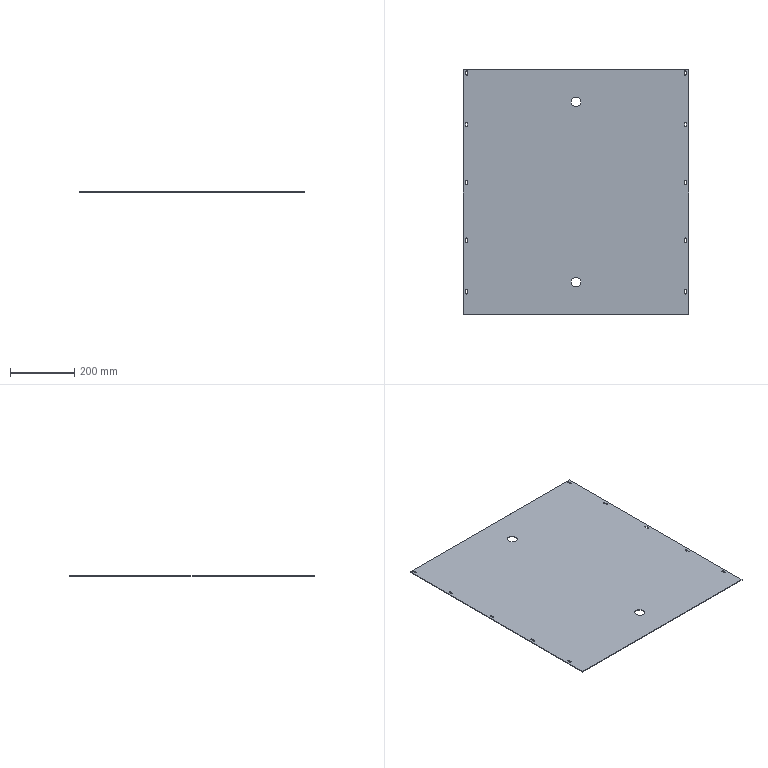Part | SolidWorks | features Cut 1, Extrusion 1, ICE 1 | 1 solid | 50 faces | box 700 x 760 x 2 mm | volume 1059954 mm3 | plane 26 | cylinder 24 | commonest cylinder face diameters 4.5 x20 30 x4